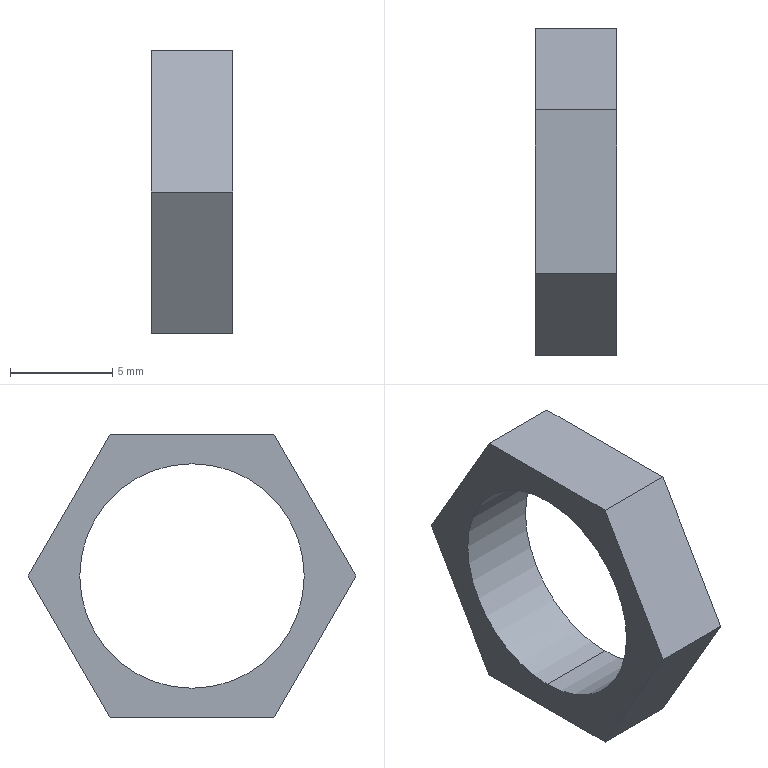Part | SolidWorks | features BaseBody 1 | 1 solid | 10 faces | box 4 x 16.062 x 13.91 mm | volume 290.13 mm3 | plane 8 | cylinder 2 | commonest cylinder face diameters 11 x2
STEP:
#1=CARTESIAN_POINT('',(324.35,123.5,18.));
#2=VERTEX_POINT('',#1);
#3=CARTESIAN_POINT('',(324.35,123.5,29.));
#4=VERTEX_POINT('',#3);
#5=CARTESIAN_POINT('',(324.35,123.5,23.5));
#6=DIRECTION('',(-1.,0.,0.));
#7=DIRECTION('',(0.,0.,1.));
#8=AXIS2_PLACEMENT_3D('',#5,#6,#7);
#9=CIRCLE('',#8,5.5);
#10=EDGE_CURVE('',#2,#4,#9,.T.);
#11=ORIENTED_EDGE('',*,*,#10,.F.);
#12=CARTESIAN_POINT('',(320.35,123.5,18.));
#13=VERTEX_POINT('',#12);
#14=CARTESIAN_POINT('',(324.35,123.5,18.));
#15=DIRECTION('',(-1.,0.,0.));
#16=VECTOR('',#15,1000.);
#17=LINE('',#14,#16);
#18=EDGE_CURVE('',#2,#13,#17,.T.);
#19=ORIENTED_EDGE('',*,*,#18,.T.);
#20=CARTESIAN_POINT('',(320.35,123.5,29.));
#21=VERTEX_POINT('',#20);
#22=CARTESIAN_POINT('',(320.35,123.5,23.5));
#23=DIRECTION('',(1.,0.,0.));
#24=DIRECTION('',(0.,0.,1.));
#25=AXIS2_PLACEMENT_3D('',#22,#23,#24);
#26=CIRCLE('',#25,5.5);
#27=EDGE_CURVE('',#21,#13,#26,.T.);
#28=ORIENTED_EDGE('',*,*,#27,.F.);
#29=CARTESIAN_POINT('',(324.35,123.5,29.));
#30=DIRECTION('',(-1.,0.,0.));
#31=VECTOR('',#30,1000.);
#32=LINE('',#29,#31);
#33=EDGE_CURVE('',#4,#21,#32,.T.);
#34=ORIENTED_EDGE('',*,*,#33,.F.);
#35=EDGE_LOOP('',(#11,#19,#28,#34));
#36=FACE_OUTER_BOUND('',#35,.T.);
#37=CARTESIAN_POINT('',(324.35,123.5,23.5));
#38=DIRECTION('',(-1.,0.,0.));
#39=DIRECTION('',(0.,0.,1.));
#40=AXIS2_PLACEMENT_3D('',#37,#38,#39);
#41=CYLINDRICAL_SURFACE('',#40,5.5);
#42=ADVANCED_FACE('',(#36),#41,.F.);
#43=ORIENTED_EDGE('',*,*,#27,.T.);
#44=CARTESIAN_POINT('',(320.35,123.5,23.5));
#45=DIRECTION('',(1.,0.,0.));
#46=DIRECTION('',(0.,0.,1.));
#47=AXIS2_PLACEMENT_3D('',#44,#45,#46);
#48=CIRCLE('',#47,5.5);
#49=EDGE_CURVE('',#13,#21,#48,.T.);
#50=ORIENTED_EDGE('',*,*,#49,.T.);
#51=EDGE_LOOP('',(#43,#50));
#52=FACE_BOUND('',#51,.T.);
#53=CARTESIAN_POINT('',(320.35,131.531,23.5));
#54=VERTEX_POINT('',#53);
#55=CARTESIAN_POINT('',(320.35,127.515,16.545));
#56=VERTEX_POINT('',#55);
#57=CARTESIAN_POINT('',(320.35,127.515,16.545));
#58=DIRECTION('',(0.,-0.5,-0.866));
#59=VECTOR('',#58,1000.);
#60=LINE('',#57,#59);
#61=EDGE_CURVE('',#54,#56,#60,.T.);
#62=ORIENTED_EDGE('',*,*,#61,.T.);
#63=CARTESIAN_POINT('',(320.35,119.485,16.545));
#64=VERTEX_POINT('',#63);
#65=CARTESIAN_POINT('',(320.35,127.515,16.545));
#66=DIRECTION('',(0.,1.,0.));
#67=VECTOR('',#66,1000.);
#68=LINE('',#65,#67);
#69=EDGE_CURVE('',#64,#56,#68,.T.);
#70=ORIENTED_EDGE('',*,*,#69,.F.);
#71=CARTESIAN_POINT('',(320.35,115.469,23.5));
#72=VERTEX_POINT('',#71);
#73=CARTESIAN_POINT('',(320.35,115.469,23.5));
#74=DIRECTION('',(0.,-0.5,0.866));
#75=VECTOR('',#74,1000.);
#76=LINE('',#73,#75);
#77=EDGE_CURVE('',#64,#72,#76,.T.);
#78=ORIENTED_EDGE('',*,*,#77,.T.);
#79=CARTESIAN_POINT('',(320.35,119.485,30.455));
#80=VERTEX_POINT('',#79);
#81=CARTESIAN_POINT('',(320.35,119.485,30.455));
#82=DIRECTION('',(0.,0.5,0.866));
#83=VECTOR('',#82,1000.);
#84=LINE('',#81,#83);
#85=EDGE_CURVE('',#72,#80,#84,.T.);
#86=ORIENTED_EDGE('',*,*,#85,.T.);
#87=CARTESIAN_POINT('',(320.35,127.515,30.455));
#88=VERTEX_POINT('',#87);
#89=CARTESIAN_POINT('',(320.35,119.485,30.455));
#90=DIRECTION('',(0.,-1.,0.));
#91=VECTOR('',#90,1000.);
#92=LINE('',#89,#91);
#93=EDGE_CURVE('',#88,#80,#92,.T.);
#94=ORIENTED_EDGE('',*,*,#93,.F.);
#95=CARTESIAN_POINT('',(320.35,131.531,23.5));
#96=DIRECTION('',(0.,0.5,-0.866));
#97=VECTOR('',#96,1000.);
#98=LINE('',#95,#97);
#99=EDGE_CURVE('',#88,#54,#98,.T.);
#100=ORIENTED_EDGE('',*,*,#99,.T.);
#101=EDGE_LOOP('',(#62,#70,#78,#86,#94,#100));
#102=FACE_OUTER_BOUND('',#101,.T.);
#103=CARTESIAN_POINT('',(320.35,123.5,23.5));
#104=DIRECTION('',(1.,0.,0.));
#105=DIRECTION('',(0.,1.,0.));
#106=AXIS2_PLACEMENT_3D('',#103,#104,#105);
#107=PLANE('',#106);
#108=ADVANCED_FACE('',(#52,#102),#107,.F.);
#109=CARTESIAN_POINT('',(324.35,127.515,16.545));
#110=VERTEX_POINT('',#109);
#111=CARTESIAN_POINT('',(324.35,131.531,23.5));
#112=VERTEX_POINT('',#111);
#113=CARTESIAN_POINT('',(324.35,127.515,16.545));
#114=DIRECTION('',(0.,0.5,0.866));
#115=VECTOR('',#114,1000.);
#116=LINE('',#113,#115);
#117=EDGE_CURVE('',#110,#112,#116,.T.);
#118=ORIENTED_EDGE('',*,*,#117,.F.);
#119=CARTESIAN_POINT('',(324.35,127.515,16.545));
#120=DIRECTION('',(1.,0.,0.));
#121=VECTOR('',#120,1000.);
#122=LINE('',#119,#121);
#123=EDGE_CURVE('',#56,#110,#122,.T.);
#124=ORIENTED_EDGE('',*,*,#123,.F.);
#125=ORIENTED_EDGE('',*,*,#61,.F.);
#126=CARTESIAN_POINT('',(324.35,131.531,23.5));
#127=DIRECTION('',(1.,0.,0.));
#128=VECTOR('',#127,1000.);
#129=LINE('',#126,#128);
#130=EDGE_CURVE('',#54,#112,#129,.T.);
#131=ORIENTED_EDGE('',*,*,#130,.T.);
#132=EDGE_LOOP('',(#118,#124,#125,#131));
#133=FACE_OUTER_BOUND('',#132,.T.);
#134=CARTESIAN_POINT('',(324.35,127.515,16.545));
#135=DIRECTION('',(0.,-0.866,0.5));
#136=DIRECTION('',(-1.,0.,0.));
#137=AXIS2_PLACEMENT_3D('',#134,#135,#136);
#138=PLANE('',#137);
#139=ADVANCED_FACE('',(#133),#138,.F.);
#140=CARTESIAN_POINT('',(324.35,127.515,30.455));
#141=VERTEX_POINT('',#140);
#142=CARTESIAN_POINT('',(324.35,131.531,23.5));
#143=DIRECTION('',(0.,-0.5,0.866));
#144=VECTOR('',#143,1000.);
#145=LINE('',#142,#144);
#146=EDGE_CURVE('',#112,#141,#145,.T.);
#147=ORIENTED_EDGE('',*,*,#146,.F.);
#148=ORIENTED_EDGE('',*,*,#130,.F.);
#149=ORIENTED_EDGE('',*,*,#99,.F.);
#150=CARTESIAN_POINT('',(324.35,127.515,30.455));
#151=DIRECTION('',(-1.,0.,0.));
#152=VECTOR('',#151,1000.);
#153=LINE('',#150,#152);
#154=EDGE_CURVE('',#141,#88,#153,.T.);
#155=ORIENTED_EDGE('',*,*,#154,.F.);
#156=EDGE_LOOP('',(#147,#148,#149,#155));
#157=FACE_OUTER_BOUND('',#156,.T.);
#158=CARTESIAN_POINT('',(324.35,131.531,23.5));
#159=DIRECTION('',(0.,-0.866,-0.5));
#160=DIRECTION('',(0.,0.5,-0.866));
#161=AXIS2_PLACEMENT_3D('',#158,#159,#160);
#162=PLANE('',#161);
#163=ADVANCED_FACE('',(#157),#162,.F.);
#164=ORIENTED_EDGE('',*,*,#93,.T.);
#165=CARTESIAN_POINT('',(324.35,119.485,30.455));
#166=VERTEX_POINT('',#165);
#167=CARTESIAN_POINT('',(324.35,119.485,30.455));
#168=DIRECTION('',(1.,0.,0.));
#169=VECTOR('',#168,1000.);
#170=LINE('',#167,#169);
#171=EDGE_CURVE('',#80,#166,#170,.T.);
#172=ORIENTED_EDGE('',*,*,#171,.T.);
#173=CARTESIAN_POINT('',(324.35,123.5,30.455));
#174=DIRECTION('',(0.,-1.,0.));
#175=VECTOR('',#174,1000.);
#176=LINE('',#173,#175);
#177=EDGE_CURVE('',#141,#166,#176,.T.);
#178=ORIENTED_EDGE('',*,*,#177,.F.);
#179=ORIENTED_EDGE('',*,*,#154,.T.);
#180=EDGE_LOOP('',(#164,#172,#178,#179));
#181=FACE_OUTER_BOUND('',#180,.T.);
#182=CARTESIAN_POINT('',(324.35,119.485,30.455));
#183=DIRECTION('',(0.,0.,1.));
#184=DIRECTION('',(0.,-1.,0.));
#185=AXIS2_PLACEMENT_3D('',#182,#183,#184);
#186=PLANE('',#185);
#187=ADVANCED_FACE('',(#181),#186,.T.);
#188=CARTESIAN_POINT('',(324.35,115.469,23.5));
#189=VERTEX_POINT('',#188);
#190=CARTESIAN_POINT('',(324.35,119.485,30.455));
#191=DIRECTION('',(0.,-0.5,-0.866));
#192=VECTOR('',#191,1000.);
#193=LINE('',#190,#192);
#194=EDGE_CURVE('',#166,#189,#193,.T.);
#195=ORIENTED_EDGE('',*,*,#194,.F.);
#196=ORIENTED_EDGE('',*,*,#171,.F.);
#197=ORIENTED_EDGE('',*,*,#85,.F.);
#198=CARTESIAN_POINT('',(324.35,115.469,23.5));
#199=DIRECTION('',(1.,0.,0.));
#200=VECTOR('',#199,1000.);
#201=LINE('',#198,#200);
#202=EDGE_CURVE('',#72,#189,#201,.T.);
#203=ORIENTED_EDGE('',*,*,#202,.T.);
#204=EDGE_LOOP('',(#195,#196,#197,#203));
#205=FACE_OUTER_BOUND('',#204,.T.);
#206=CARTESIAN_POINT('',(324.35,119.485,30.455));
#207=DIRECTION('',(0.,0.866,-0.5));
#208=DIRECTION('',(-1.,0.,0.));
#209=AXIS2_PLACEMENT_3D('',#206,#207,#208);
#210=PLANE('',#209);
#211=ADVANCED_FACE('',(#205),#210,.F.);
#212=CARTESIAN_POINT('',(324.35,119.485,16.545));
#213=VERTEX_POINT('',#212);
#214=CARTESIAN_POINT('',(324.35,115.469,23.5));
#215=DIRECTION('',(0.,0.5,-0.866));
#216=VECTOR('',#215,1000.);
#217=LINE('',#214,#216);
#218=EDGE_CURVE('',#189,#213,#217,.T.);
#219=ORIENTED_EDGE('',*,*,#218,.F.);
#220=ORIENTED_EDGE('',*,*,#202,.F.);
#221=ORIENTED_EDGE('',*,*,#77,.F.);
#222=CARTESIAN_POINT('',(324.35,119.485,16.545));
#223=DIRECTION('',(-1.,0.,0.));
#224=VECTOR('',#223,1000.);
#225=LINE('',#222,#224);
#226=EDGE_CURVE('',#213,#64,#225,.T.);
#227=ORIENTED_EDGE('',*,*,#226,.F.);
#228=EDGE_LOOP('',(#219,#220,#221,#227));
#229=FACE_OUTER_BOUND('',#228,.T.);
#230=CARTESIAN_POINT('',(324.35,115.469,23.5));
#231=DIRECTION('',(0.,0.866,0.5));
#232=DIRECTION('',(1.,0.,0.));
#233=AXIS2_PLACEMENT_3D('',#230,#231,#232);
#234=PLANE('',#233);
#235=ADVANCED_FACE('',(#229),#234,.F.);
#236=ORIENTED_EDGE('',*,*,#69,.T.);
#237=ORIENTED_EDGE('',*,*,#123,.T.);
#238=CARTESIAN_POINT('',(324.35,123.5,16.545));
#239=DIRECTION('',(0.,1.,0.));
#240=VECTOR('',#239,1000.);
#241=LINE('',#238,#240);
#242=EDGE_CURVE('',#213,#110,#241,.T.);
#243=ORIENTED_EDGE('',*,*,#242,.F.);
#244=ORIENTED_EDGE('',*,*,#226,.T.);
#245=EDGE_LOOP('',(#236,#237,#243,#244));
#246=FACE_OUTER_BOUND('',#245,.T.);
#247=CARTESIAN_POINT('',(324.35,127.515,16.545));
#248=DIRECTION('',(0.,0.,-1.));
#249=DIRECTION('',(0.,-1.,0.));
#250=AXIS2_PLACEMENT_3D('',#247,#248,#249);
#251=PLANE('',#250);
#252=ADVANCED_FACE('',(#246),#251,.T.);
#253=CARTESIAN_POINT('',(324.35,123.5,23.5));
#254=DIRECTION('',(-1.,0.,0.));
#255=DIRECTION('',(0.,0.,1.));
#256=AXIS2_PLACEMENT_3D('',#253,#254,#255);
#257=CIRCLE('',#256,5.5);
#258=EDGE_CURVE('',#4,#2,#257,.T.);
#259=ORIENTED_EDGE('',*,*,#258,.T.);
#260=ORIENTED_EDGE('',*,*,#10,.T.);
#261=EDGE_LOOP('',(#259,#260));
#262=FACE_BOUND('',#261,.T.);
#263=ORIENTED_EDGE('',*,*,#218,.T.);
#264=ORIENTED_EDGE('',*,*,#242,.T.);
#265=ORIENTED_EDGE('',*,*,#117,.T.);
#266=ORIENTED_EDGE('',*,*,#146,.T.);
#267=ORIENTED_EDGE('',*,*,#177,.T.);
#268=ORIENTED_EDGE('',*,*,#194,.T.);
#269=EDGE_LOOP('',(#263,#264,#265,#266,#267,#268));
#270=FACE_OUTER_BOUND('',#269,.T.);
#271=CARTESIAN_POINT('',(324.35,123.5,23.5));
#272=DIRECTION('',(1.,0.,0.));
#273=DIRECTION('',(0.,1.,0.));
#274=AXIS2_PLACEMENT_3D('',#271,#272,#273);
#275=PLANE('',#274);
#276=ADVANCED_FACE('',(#262,#270),#275,.T.);
#277=ORIENTED_EDGE('',*,*,#18,.F.);
#278=ORIENTED_EDGE('',*,*,#258,.F.);
#279=ORIENTED_EDGE('',*,*,#33,.T.);
#280=ORIENTED_EDGE('',*,*,#49,.F.);
#281=EDGE_LOOP('',(#277,#278,#279,#280));
#282=FACE_OUTER_BOUND('',#281,.T.);
#283=CARTESIAN_POINT('',(324.35,123.5,23.5));
#284=DIRECTION('',(-1.,0.,0.));
#285=DIRECTION('',(0.,0.,1.));
#286=AXIS2_PLACEMENT_3D('',#283,#284,#285);
#287=CYLINDRICAL_SURFACE('',#286,5.5);
#288=ADVANCED_FACE('',(#282),#287,.F.);
#289=CLOSED_SHELL('',(#42,#108,#139,#163,#187,#211,#235,#252,#276,#288));
#290=MANIFOLD_SOLID_BREP('',#289);
#291=CARTESIAN_POINT('',(0.,0.,0.));
#292=DIRECTION('',(0.,0.,1.));
#293=DIRECTION('',(1.,0.,0.));
#294=AXIS2_PLACEMENT_3D('',#291,#292,#293);
#295=(LENGTH_UNIT()NAMED_UNIT(*)SI_UNIT(.MILLI.,.METRE.));
#296=UNCERTAINTY_MEASURE_WITH_UNIT(LENGTH_MEASURE(0.00001),#295,'','');
#297=(NAMED_UNIT(*)PLANE_ANGLE_UNIT()SI_UNIT($,.RADIAN.));
#298=(NAMED_UNIT(*)SI_UNIT($,.STERADIAN.)SOLID_ANGLE_UNIT());
#299=(GEOMETRIC_REPRESENTATION_CONTEXT(3)GLOBAL_UNCERTAINTY_ASSIGNED_CONTEXT((#296))GLOBAL_UNIT_ASSIGNED_CONTEXT((#295,#297,#298))REPRESENTATION_CONTEXT('',''));
#300=ADVANCED_BREP_SHAPE_REPRESENTATION('',(#290,#294),#299);